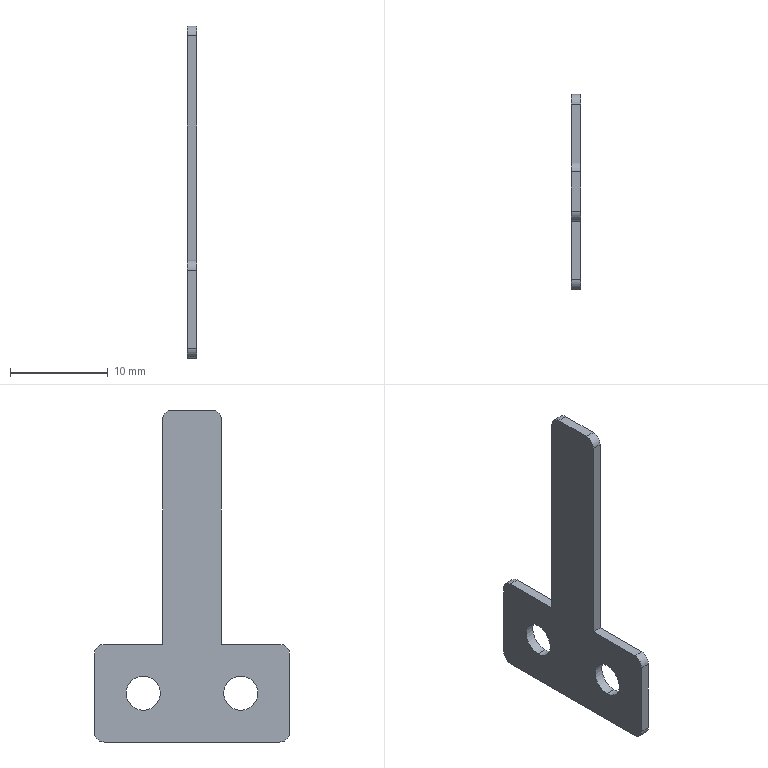Part | SolidWorks | features BaseBody 1 | 1 solid | 20 faces | box 1 x 20 x 34 mm | volume 323.47 mm3 | cylinder 10 | plane 10 | commonest cylinder face diameters 2 x6 3.5 x4
STEP:
#1=CARTESIAN_POINT('',(-1.,10.,-16.));
#2=VERTEX_POINT('',#1);
#3=CARTESIAN_POINT('',(-1.,9.,-17.));
#4=VERTEX_POINT('',#3);
#5=CARTESIAN_POINT('',(-1.,9.,-16.));
#6=DIRECTION('',(-1.,0.,0.));
#7=DIRECTION('',(0.,0.,-1.));
#8=AXIS2_PLACEMENT_3D('',#5,#6,#7);
#9=CIRCLE('',#8,1.);
#10=EDGE_CURVE('',#2,#4,#9,.T.);
#11=ORIENTED_EDGE('',*,*,#10,.F.);
#12=CARTESIAN_POINT('',(0.,10.,-16.));
#13=VERTEX_POINT('',#12);
#14=CARTESIAN_POINT('',(0.,10.,-16.));
#15=DIRECTION('',(-1.,0.,0.));
#16=VECTOR('',#15,1000.);
#17=LINE('',#14,#16);
#18=EDGE_CURVE('',#13,#2,#17,.T.);
#19=ORIENTED_EDGE('',*,*,#18,.F.);
#20=CARTESIAN_POINT('',(0.,9.,-17.));
#21=VERTEX_POINT('',#20);
#22=CARTESIAN_POINT('',(0.,9.,-16.));
#23=DIRECTION('',(1.,0.,0.));
#24=DIRECTION('',(0.,0.,-1.));
#25=AXIS2_PLACEMENT_3D('',#22,#23,#24);
#26=CIRCLE('',#25,1.);
#27=EDGE_CURVE('',#21,#13,#26,.T.);
#28=ORIENTED_EDGE('',*,*,#27,.F.);
#29=CARTESIAN_POINT('',(-1.,9.,-17.));
#30=DIRECTION('',(1.,0.,0.));
#31=VECTOR('',#30,1000.);
#32=LINE('',#29,#31);
#33=EDGE_CURVE('',#4,#21,#32,.T.);
#34=ORIENTED_EDGE('',*,*,#33,.F.);
#35=EDGE_LOOP('',(#11,#19,#28,#34));
#36=FACE_OUTER_BOUND('',#35,.T.);
#37=CARTESIAN_POINT('',(-1.,9.,-16.));
#38=DIRECTION('',(1.,0.,0.));
#39=DIRECTION('',(0.,0.,-1.));
#40=AXIS2_PLACEMENT_3D('',#37,#38,#39);
#41=CYLINDRICAL_SURFACE('',#40,1.);
#42=ADVANCED_FACE('',(#36),#41,.T.);
#43=CARTESIAN_POINT('',(-1.,9.,-7.));
#44=VERTEX_POINT('',#43);
#45=CARTESIAN_POINT('',(-1.,10.,-8.));
#46=VERTEX_POINT('',#45);
#47=CARTESIAN_POINT('',(-1.,9.,-8.));
#48=DIRECTION('',(-1.,0.,0.));
#49=DIRECTION('',(0.,0.,-1.));
#50=AXIS2_PLACEMENT_3D('',#47,#48,#49);
#51=CIRCLE('',#50,1.);
#52=EDGE_CURVE('',#44,#46,#51,.T.);
#53=ORIENTED_EDGE('',*,*,#52,.F.);
#54=CARTESIAN_POINT('',(0.,9.,-7.));
#55=VERTEX_POINT('',#54);
#56=CARTESIAN_POINT('',(-1.,9.,-7.));
#57=DIRECTION('',(-1.,0.,0.));
#58=VECTOR('',#57,1000.);
#59=LINE('',#56,#58);
#60=EDGE_CURVE('',#55,#44,#59,.T.);
#61=ORIENTED_EDGE('',*,*,#60,.F.);
#62=CARTESIAN_POINT('',(0.,10.,-8.));
#63=VERTEX_POINT('',#62);
#64=CARTESIAN_POINT('',(0.,9.,-8.));
#65=DIRECTION('',(1.,0.,0.));
#66=DIRECTION('',(0.,0.,-1.));
#67=AXIS2_PLACEMENT_3D('',#64,#65,#66);
#68=CIRCLE('',#67,1.);
#69=EDGE_CURVE('',#63,#55,#68,.T.);
#70=ORIENTED_EDGE('',*,*,#69,.F.);
#71=CARTESIAN_POINT('',(0.,10.,-8.));
#72=DIRECTION('',(1.,0.,0.));
#73=VECTOR('',#72,1000.);
#74=LINE('',#71,#73);
#75=EDGE_CURVE('',#46,#63,#74,.T.);
#76=ORIENTED_EDGE('',*,*,#75,.F.);
#77=EDGE_LOOP('',(#53,#61,#70,#76));
#78=FACE_OUTER_BOUND('',#77,.T.);
#79=CARTESIAN_POINT('',(0.,9.,-8.));
#80=DIRECTION('',(-1.,0.,0.));
#81=DIRECTION('',(0.,0.,1.));
#82=AXIS2_PLACEMENT_3D('',#79,#80,#81);
#83=CYLINDRICAL_SURFACE('',#82,1.);
#84=ADVANCED_FACE('',(#78),#83,.T.);
#85=CARTESIAN_POINT('',(-1.,2.,17.));
#86=VERTEX_POINT('',#85);
#87=CARTESIAN_POINT('',(-1.,3.,16.));
#88=VERTEX_POINT('',#87);
#89=CARTESIAN_POINT('',(-1.,2.,16.));
#90=DIRECTION('',(-1.,0.,0.));
#91=DIRECTION('',(0.,0.,-1.));
#92=AXIS2_PLACEMENT_3D('',#89,#90,#91);
#93=CIRCLE('',#92,1.);
#94=EDGE_CURVE('',#86,#88,#93,.T.);
#95=ORIENTED_EDGE('',*,*,#94,.F.);
#96=CARTESIAN_POINT('',(0.,2.,17.));
#97=VERTEX_POINT('',#96);
#98=CARTESIAN_POINT('',(-1.,2.,17.));
#99=DIRECTION('',(-1.,0.,0.));
#100=VECTOR('',#99,1000.);
#101=LINE('',#98,#100);
#102=EDGE_CURVE('',#97,#86,#101,.T.);
#103=ORIENTED_EDGE('',*,*,#102,.F.);
#104=CARTESIAN_POINT('',(0.,3.,16.));
#105=VERTEX_POINT('',#104);
#106=CARTESIAN_POINT('',(0.,2.,16.));
#107=DIRECTION('',(1.,0.,0.));
#108=DIRECTION('',(0.,0.,-1.));
#109=AXIS2_PLACEMENT_3D('',#106,#107,#108);
#110=CIRCLE('',#109,1.);
#111=EDGE_CURVE('',#105,#97,#110,.T.);
#112=ORIENTED_EDGE('',*,*,#111,.F.);
#113=CARTESIAN_POINT('',(0.,3.,16.));
#114=DIRECTION('',(1.,0.,0.));
#115=VECTOR('',#114,1000.);
#116=LINE('',#113,#115);
#117=EDGE_CURVE('',#88,#105,#116,.T.);
#118=ORIENTED_EDGE('',*,*,#117,.F.);
#119=EDGE_LOOP('',(#95,#103,#112,#118));
#120=FACE_OUTER_BOUND('',#119,.T.);
#121=CARTESIAN_POINT('',(-26.,2.,16.));
#122=DIRECTION('',(-1.,0.,0.));
#123=DIRECTION('',(0.,0.,1.));
#124=AXIS2_PLACEMENT_3D('',#121,#122,#123);
#125=CYLINDRICAL_SURFACE('',#124,1.);
#126=ADVANCED_FACE('',(#120),#125,.T.);
#127=CARTESIAN_POINT('',(-1.,-3.,16.));
#128=VERTEX_POINT('',#127);
#129=CARTESIAN_POINT('',(-1.,-2.,17.));
#130=VERTEX_POINT('',#129);
#131=CARTESIAN_POINT('',(-1.,-2.,16.));
#132=DIRECTION('',(-1.,0.,0.));
#133=DIRECTION('',(0.,0.,-1.));
#134=AXIS2_PLACEMENT_3D('',#131,#132,#133);
#135=CIRCLE('',#134,1.);
#136=EDGE_CURVE('',#128,#130,#135,.T.);
#137=ORIENTED_EDGE('',*,*,#136,.F.);
#138=CARTESIAN_POINT('',(0.,-3.,16.));
#139=VERTEX_POINT('',#138);
#140=CARTESIAN_POINT('',(-1.,-3.,16.));
#141=DIRECTION('',(-1.,0.,0.));
#142=VECTOR('',#141,1000.);
#143=LINE('',#140,#142);
#144=EDGE_CURVE('',#139,#128,#143,.T.);
#145=ORIENTED_EDGE('',*,*,#144,.F.);
#146=CARTESIAN_POINT('',(0.,-2.,17.));
#147=VERTEX_POINT('',#146);
#148=CARTESIAN_POINT('',(0.,-2.,16.));
#149=DIRECTION('',(1.,0.,0.));
#150=DIRECTION('',(0.,0.,-1.));
#151=AXIS2_PLACEMENT_3D('',#148,#149,#150);
#152=CIRCLE('',#151,1.);
#153=EDGE_CURVE('',#147,#139,#152,.T.);
#154=ORIENTED_EDGE('',*,*,#153,.F.);
#155=CARTESIAN_POINT('',(0.,-2.,17.));
#156=DIRECTION('',(1.,0.,0.));
#157=VECTOR('',#156,1000.);
#158=LINE('',#155,#157);
#159=EDGE_CURVE('',#130,#147,#158,.T.);
#160=ORIENTED_EDGE('',*,*,#159,.F.);
#161=EDGE_LOOP('',(#137,#145,#154,#160));
#162=FACE_OUTER_BOUND('',#161,.T.);
#163=CARTESIAN_POINT('',(0.,-2.,16.));
#164=DIRECTION('',(-1.,0.,0.));
#165=DIRECTION('',(0.,0.,1.));
#166=AXIS2_PLACEMENT_3D('',#163,#164,#165);
#167=CYLINDRICAL_SURFACE('',#166,1.);
#168=ADVANCED_FACE('',(#162),#167,.T.);
#169=CARTESIAN_POINT('',(-1.,-10.,-8.));
#170=VERTEX_POINT('',#169);
#171=CARTESIAN_POINT('',(-1.,-9.,-7.));
#172=VERTEX_POINT('',#171);
#173=CARTESIAN_POINT('',(-1.,-9.,-8.));
#174=DIRECTION('',(-1.,0.,0.));
#175=DIRECTION('',(0.,0.,-1.));
#176=AXIS2_PLACEMENT_3D('',#173,#174,#175);
#177=CIRCLE('',#176,1.);
#178=EDGE_CURVE('',#170,#172,#177,.T.);
#179=ORIENTED_EDGE('',*,*,#178,.F.);
#180=CARTESIAN_POINT('',(0.,-10.,-8.));
#181=VERTEX_POINT('',#180);
#182=CARTESIAN_POINT('',(0.,-10.,-8.));
#183=DIRECTION('',(-1.,0.,0.));
#184=VECTOR('',#183,1000.);
#185=LINE('',#182,#184);
#186=EDGE_CURVE('',#181,#170,#185,.T.);
#187=ORIENTED_EDGE('',*,*,#186,.F.);
#188=CARTESIAN_POINT('',(0.,-9.,-7.));
#189=VERTEX_POINT('',#188);
#190=CARTESIAN_POINT('',(0.,-9.,-8.));
#191=DIRECTION('',(1.,0.,0.));
#192=DIRECTION('',(0.,0.,-1.));
#193=AXIS2_PLACEMENT_3D('',#190,#191,#192);
#194=CIRCLE('',#193,1.);
#195=EDGE_CURVE('',#189,#181,#194,.T.);
#196=ORIENTED_EDGE('',*,*,#195,.F.);
#197=CARTESIAN_POINT('',(-26.,-9.,-7.));
#198=DIRECTION('',(1.,0.,0.));
#199=VECTOR('',#198,1000.);
#200=LINE('',#197,#199);
#201=EDGE_CURVE('',#172,#189,#200,.T.);
#202=ORIENTED_EDGE('',*,*,#201,.F.);
#203=EDGE_LOOP('',(#179,#187,#196,#202));
#204=FACE_OUTER_BOUND('',#203,.T.);
#205=CARTESIAN_POINT('',(-26.,-9.,-8.));
#206=DIRECTION('',(1.,0.,0.));
#207=DIRECTION('',(0.,0.,-1.));
#208=AXIS2_PLACEMENT_3D('',#205,#206,#207);
#209=CYLINDRICAL_SURFACE('',#208,1.);
#210=ADVANCED_FACE('',(#204),#209,.T.);
#211=CARTESIAN_POINT('',(-1.,-9.,-17.));
#212=VERTEX_POINT('',#211);
#213=CARTESIAN_POINT('',(-1.,-10.,-16.));
#214=VERTEX_POINT('',#213);
#215=CARTESIAN_POINT('',(-1.,-9.,-16.));
#216=DIRECTION('',(-1.,0.,0.));
#217=DIRECTION('',(0.,0.,-1.));
#218=AXIS2_PLACEMENT_3D('',#215,#216,#217);
#219=CIRCLE('',#218,1.);
#220=EDGE_CURVE('',#212,#214,#219,.T.);
#221=ORIENTED_EDGE('',*,*,#220,.F.);
#222=CARTESIAN_POINT('',(0.,-9.,-17.));
#223=VERTEX_POINT('',#222);
#224=CARTESIAN_POINT('',(-1.,-9.,-17.));
#225=DIRECTION('',(-1.,0.,0.));
#226=VECTOR('',#225,1000.);
#227=LINE('',#224,#226);
#228=EDGE_CURVE('',#223,#212,#227,.T.);
#229=ORIENTED_EDGE('',*,*,#228,.F.);
#230=CARTESIAN_POINT('',(0.,-10.,-16.));
#231=VERTEX_POINT('',#230);
#232=CARTESIAN_POINT('',(0.,-9.,-16.));
#233=DIRECTION('',(1.,0.,0.));
#234=DIRECTION('',(0.,0.,-1.));
#235=AXIS2_PLACEMENT_3D('',#232,#233,#234);
#236=CIRCLE('',#235,1.);
#237=EDGE_CURVE('',#231,#223,#236,.T.);
#238=ORIENTED_EDGE('',*,*,#237,.F.);
#239=CARTESIAN_POINT('',(0.,-10.,-16.));
#240=DIRECTION('',(1.,0.,0.));
#241=VECTOR('',#240,1000.);
#242=LINE('',#239,#241);
#243=EDGE_CURVE('',#214,#231,#242,.T.);
#244=ORIENTED_EDGE('',*,*,#243,.F.);
#245=EDGE_LOOP('',(#221,#229,#238,#244));
#246=FACE_OUTER_BOUND('',#245,.T.);
#247=CARTESIAN_POINT('',(0.,-9.,-16.));
#248=DIRECTION('',(-1.,0.,0.));
#249=DIRECTION('',(0.,0.,1.));
#250=AXIS2_PLACEMENT_3D('',#247,#248,#249);
#251=CYLINDRICAL_SURFACE('',#250,1.);
#252=ADVANCED_FACE('',(#246),#251,.T.);
#253=CARTESIAN_POINT('',(-1.,3.,-7.));
#254=VERTEX_POINT('',#253);
#255=CARTESIAN_POINT('',(-1.,3.,17.));
#256=DIRECTION('',(0.,0.,1.));
#257=VECTOR('',#256,1000.);
#258=LINE('',#255,#257);
#259=EDGE_CURVE('',#254,#88,#258,.T.);
#260=ORIENTED_EDGE('',*,*,#259,.T.);
#261=ORIENTED_EDGE('',*,*,#117,.T.);
#262=CARTESIAN_POINT('',(0.,3.,-7.));
#263=VERTEX_POINT('',#262);
#264=CARTESIAN_POINT('',(0.,3.,17.));
#265=DIRECTION('',(0.,0.,-1.));
#266=VECTOR('',#265,1000.);
#267=LINE('',#264,#266);
#268=EDGE_CURVE('',#105,#263,#267,.T.);
#269=ORIENTED_EDGE('',*,*,#268,.T.);
#270=CARTESIAN_POINT('',(-26.,3.,-7.));
#271=DIRECTION('',(1.,0.,0.));
#272=VECTOR('',#271,1000.);
#273=LINE('',#270,#272);
#274=EDGE_CURVE('',#254,#263,#273,.T.);
#275=ORIENTED_EDGE('',*,*,#274,.F.);
#276=EDGE_LOOP('',(#260,#261,#269,#275));
#277=FACE_OUTER_BOUND('',#276,.T.);
#278=CARTESIAN_POINT('',(-26.,3.,17.));
#279=DIRECTION('',(0.,-1.,0.));
#280=DIRECTION('',(0.,0.,-1.));
#281=AXIS2_PLACEMENT_3D('',#278,#279,#280);
#282=PLANE('',#281);
#283=ADVANCED_FACE('',(#277),#282,.F.);
#284=CARTESIAN_POINT('',(0.,10.,-7.));
#285=DIRECTION('',(0.,1.,0.));
#286=VECTOR('',#285,1000.);
#287=LINE('',#284,#286);
#288=EDGE_CURVE('',#263,#55,#287,.T.);
#289=ORIENTED_EDGE('',*,*,#288,.T.);
#290=ORIENTED_EDGE('',*,*,#60,.T.);
#291=CARTESIAN_POINT('',(-1.,10.,-7.));
#292=DIRECTION('',(0.,-1.,0.));
#293=VECTOR('',#292,1000.);
#294=LINE('',#291,#293);
#295=EDGE_CURVE('',#44,#254,#294,.T.);
#296=ORIENTED_EDGE('',*,*,#295,.T.);
#297=ORIENTED_EDGE('',*,*,#274,.T.);
#298=EDGE_LOOP('',(#289,#290,#296,#297));
#299=FACE_OUTER_BOUND('',#298,.T.);
#300=CARTESIAN_POINT('',(-26.,10.,-7.));
#301=DIRECTION('',(0.,0.,-1.));
#302=DIRECTION('',(-1.,0.,0.));
#303=AXIS2_PLACEMENT_3D('',#300,#301,#302);
#304=PLANE('',#303);
#305=ADVANCED_FACE('',(#299),#304,.F.);
#306=CARTESIAN_POINT('',(-1.,-3.,-7.));
#307=VERTEX_POINT('',#306);
#308=CARTESIAN_POINT('',(-1.,-10.,-7.));
#309=DIRECTION('',(0.,-1.,0.));
#310=VECTOR('',#309,1000.);
#311=LINE('',#308,#310);
#312=EDGE_CURVE('',#307,#172,#311,.T.);
#313=ORIENTED_EDGE('',*,*,#312,.T.);
#314=ORIENTED_EDGE('',*,*,#201,.T.);
#315=CARTESIAN_POINT('',(0.,-3.,-7.));
#316=VERTEX_POINT('',#315);
#317=CARTESIAN_POINT('',(0.,-10.,-7.));
#318=DIRECTION('',(0.,1.,0.));
#319=VECTOR('',#318,1000.);
#320=LINE('',#317,#319);
#321=EDGE_CURVE('',#189,#316,#320,.T.);
#322=ORIENTED_EDGE('',*,*,#321,.T.);
#323=CARTESIAN_POINT('',(-26.,-3.,-7.));
#324=DIRECTION('',(1.,0.,0.));
#325=VECTOR('',#324,1000.);
#326=LINE('',#323,#325);
#327=EDGE_CURVE('',#307,#316,#326,.T.);
#328=ORIENTED_EDGE('',*,*,#327,.F.);
#329=EDGE_LOOP('',(#313,#314,#322,#328));
#330=FACE_OUTER_BOUND('',#329,.T.);
#331=CARTESIAN_POINT('',(-26.,-10.,-7.));
#332=DIRECTION('',(0.,0.,-1.));
#333=DIRECTION('',(-1.,0.,0.));
#334=AXIS2_PLACEMENT_3D('',#331,#332,#333);
#335=PLANE('',#334);
#336=ADVANCED_FACE('',(#330),#335,.F.);
#337=CARTESIAN_POINT('',(0.,-3.,17.));
#338=DIRECTION('',(0.,0.,1.));
#339=VECTOR('',#338,1000.);
#340=LINE('',#337,#339);
#341=EDGE_CURVE('',#316,#139,#340,.T.);
#342=ORIENTED_EDGE('',*,*,#341,.T.);
#343=ORIENTED_EDGE('',*,*,#144,.T.);
#344=CARTESIAN_POINT('',(-1.,-3.,17.));
#345=DIRECTION('',(0.,0.,-1.));
#346=VECTOR('',#345,1000.);
#347=LINE('',#344,#346);
#348=EDGE_CURVE('',#128,#307,#347,.T.);
#349=ORIENTED_EDGE('',*,*,#348,.T.);
#350=ORIENTED_EDGE('',*,*,#327,.T.);
#351=EDGE_LOOP('',(#342,#343,#349,#350));
#352=FACE_OUTER_BOUND('',#351,.T.);
#353=CARTESIAN_POINT('',(-26.,-3.,17.));
#354=DIRECTION('',(0.,1.,0.));
#355=DIRECTION('',(0.,0.,-1.));
#356=AXIS2_PLACEMENT_3D('',#353,#354,#355);
#357=PLANE('',#356);
#358=ADVANCED_FACE('',(#352),#357,.F.);
#359=CARTESIAN_POINT('',(-1.,5.,-10.25));
#360=VERTEX_POINT('',#359);
#361=CARTESIAN_POINT('',(0.,5.,-10.25));
#362=VERTEX_POINT('',#361);
#363=CARTESIAN_POINT('',(0.,5.,-10.25));
#364=DIRECTION('',(1.,0.,0.));
#365=VECTOR('',#364,1000.);
#366=LINE('',#363,#365);
#367=EDGE_CURVE('',#360,#362,#366,.T.);
#368=ORIENTED_EDGE('',*,*,#367,.F.);
#369=CARTESIAN_POINT('',(-1.,5.,-13.75));
#370=VERTEX_POINT('',#369);
#371=CARTESIAN_POINT('',(-1.,5.,-12.));
#372=DIRECTION('',(1.,0.,0.));
#373=DIRECTION('',(0.,0.,-1.));
#374=AXIS2_PLACEMENT_3D('',#371,#372,#373);
#375=CIRCLE('',#374,1.75);
#376=EDGE_CURVE('',#370,#360,#375,.T.);
#377=ORIENTED_EDGE('',*,*,#376,.F.);
#378=CARTESIAN_POINT('',(0.,5.,-13.75));
#379=VERTEX_POINT('',#378);
#380=CARTESIAN_POINT('',(0.,5.,-13.75));
#381=DIRECTION('',(1.,0.,0.));
#382=VECTOR('',#381,1000.);
#383=LINE('',#380,#382);
#384=EDGE_CURVE('',#370,#379,#383,.T.);
#385=ORIENTED_EDGE('',*,*,#384,.T.);
#386=CARTESIAN_POINT('',(0.,5.,-12.));
#387=DIRECTION('',(1.,0.,0.));
#388=DIRECTION('',(0.,0.,-1.));
#389=AXIS2_PLACEMENT_3D('',#386,#387,#388);
#390=CIRCLE('',#389,1.75);
#391=EDGE_CURVE('',#379,#362,#390,.T.);
#392=ORIENTED_EDGE('',*,*,#391,.T.);
#393=EDGE_LOOP('',(#368,#377,#385,#392));
#394=FACE_OUTER_BOUND('',#393,.T.);
#395=CARTESIAN_POINT('',(0.,5.,-12.));
#396=DIRECTION('',(1.,0.,0.));
#397=DIRECTION('',(0.,0.,-1.));
#398=AXIS2_PLACEMENT_3D('',#395,#396,#397);
#399=CYLINDRICAL_SURFACE('',#398,1.75);
#400=ADVANCED_FACE('',(#394),#399,.F.);
#401=CARTESIAN_POINT('',(-1.,-5.,-10.25));
#402=VERTEX_POINT('',#401);
#403=CARTESIAN_POINT('',(0.,-5.,-10.25));
#404=VERTEX_POINT('',#403);
#405=CARTESIAN_POINT('',(0.,-5.,-10.25));
#406=DIRECTION('',(1.,0.,0.));
#407=VECTOR('',#406,1000.);
#408=LINE('',#405,#407);
#409=EDGE_CURVE('',#402,#404,#408,.T.);
#410=ORIENTED_EDGE('',*,*,#409,.F.);
#411=CARTESIAN_POINT('',(-1.,-5.,-13.75));
#412=VERTEX_POINT('',#411);
#413=CARTESIAN_POINT('',(-1.,-5.,-12.));
#414=DIRECTION('',(1.,0.,0.));
#415=DIRECTION('',(0.,0.,-1.));
#416=AXIS2_PLACEMENT_3D('',#413,#414,#415);
#417=CIRCLE('',#416,1.75);
#418=EDGE_CURVE('',#412,#402,#417,.T.);
#419=ORIENTED_EDGE('',*,*,#418,.F.);
#420=CARTESIAN_POINT('',(0.,-5.,-13.75));
#421=VERTEX_POINT('',#420);
#422=CARTESIAN_POINT('',(0.,-5.,-13.75));
#423=DIRECTION('',(1.,0.,0.));
#424=VECTOR('',#423,1000.);
#425=LINE('',#422,#424);
#426=EDGE_CURVE('',#412,#421,#425,.T.);
#427=ORIENTED_EDGE('',*,*,#426,.T.);
#428=CARTESIAN_POINT('',(0.,-5.,-12.));
#429=DIRECTION('',(1.,0.,0.));
#430=DIRECTION('',(0.,0.,-1.));
#431=AXIS2_PLACEMENT_3D('',#428,#429,#430);
#432=CIRCLE('',#431,1.75);
#433=EDGE_CURVE('',#421,#404,#432,.T.);
#434=ORIENTED_EDGE('',*,*,#433,.T.);
#435=EDGE_LOOP('',(#410,#419,#427,#434));
#436=FACE_OUTER_BOUND('',#435,.T.);
#437=CARTESIAN_POINT('',(0.,-5.,-12.));
#438=DIRECTION('',(1.,0.,0.));
#439=DIRECTION('',(0.,0.,-1.));
#440=AXIS2_PLACEMENT_3D('',#437,#438,#439);
#441=CYLINDRICAL_SURFACE('',#440,1.75);
#442=ADVANCED_FACE('',(#436),#441,.F.);
#443=CARTESIAN_POINT('',(-1.,-10.,-17.));
#444=DIRECTION('',(0.,0.,1.));
#445=VECTOR('',#444,1000.);
#446=LINE('',#443,#445);
#447=EDGE_CURVE('',#214,#170,#446,.T.);
#448=ORIENTED_EDGE('',*,*,#447,.F.);
#449=ORIENTED_EDGE('',*,*,#243,.T.);
#450=CARTESIAN_POINT('',(0.,-10.,-17.));
#451=DIRECTION('',(0.,0.,1.));
#452=VECTOR('',#451,1000.);
#453=LINE('',#450,#452);
#454=EDGE_CURVE('',#231,#181,#453,.T.);
#455=ORIENTED_EDGE('',*,*,#454,.T.);
#456=ORIENTED_EDGE('',*,*,#186,.T.);
#457=EDGE_LOOP('',(#448,#449,#455,#456));
#458=FACE_OUTER_BOUND('',#457,.T.);
#459=CARTESIAN_POINT('',(0.,-10.,0.));
#460=DIRECTION('',(0.,1.,0.));
#461=DIRECTION('',(1.,0.,0.));
#462=AXIS2_PLACEMENT_3D('',#459,#460,#461);
#463=PLANE('',#462);
#464=ADVANCED_FACE('',(#458),#463,.F.);
#465=CARTESIAN_POINT('',(-1.,10.,-17.));
#466=DIRECTION('',(0.,0.,1.));
#467=VECTOR('',#466,1000.);
#468=LINE('',#465,#467);
#469=EDGE_CURVE('',#2,#46,#468,.T.);
#470=ORIENTED_EDGE('',*,*,#469,.T.);
#471=ORIENTED_EDGE('',*,*,#75,.T.);
#472=CARTESIAN_POINT('',(0.,10.,-17.));
#473=DIRECTION('',(0.,0.,1.));
#474=VECTOR('',#473,1000.);
#475=LINE('',#472,#474);
#476=EDGE_CURVE('',#13,#63,#475,.T.);
#477=ORIENTED_EDGE('',*,*,#476,.F.);
#478=ORIENTED_EDGE('',*,*,#18,.T.);
#479=EDGE_LOOP('',(#470,#471,#477,#478));
#480=FACE_OUTER_BOUND('',#479,.T.);
#481=CARTESIAN_POINT('',(0.,10.,0.));
#482=DIRECTION('',(0.,1.,0.));
#483=DIRECTION('',(1.,0.,0.));
#484=AXIS2_PLACEMENT_3D('',#481,#482,#483);
#485=PLANE('',#484);
#486=ADVANCED_FACE('',(#480),#485,.T.);
#487=CARTESIAN_POINT('',(0.,10.,-17.));
#488=DIRECTION('',(0.,-1.,0.));
#489=VECTOR('',#488,1000.);
#490=LINE('',#487,#489);
#491=EDGE_CURVE('',#21,#223,#490,.T.);
#492=ORIENTED_EDGE('',*,*,#491,.T.);
#493=ORIENTED_EDGE('',*,*,#228,.T.);
#494=CARTESIAN_POINT('',(-1.,10.,-17.));
#495=DIRECTION('',(0.,-1.,0.));
#496=VECTOR('',#495,1000.);
#497=LINE('',#494,#496);
#498=EDGE_CURVE('',#4,#212,#497,.T.);
#499=ORIENTED_EDGE('',*,*,#498,.F.);
#500=ORIENTED_EDGE('',*,*,#33,.T.);
#501=EDGE_LOOP('',(#492,#493,#499,#500));
#502=FACE_OUTER_BOUND('',#501,.T.);
#503=CARTESIAN_POINT('',(-1.,10.,-17.));
#504=DIRECTION('',(0.,0.,-1.));
#505=DIRECTION('',(0.,-1.,0.));
#506=AXIS2_PLACEMENT_3D('',#503,#504,#505);
#507=PLANE('',#506);
#508=ADVANCED_FACE('',(#502),#507,.T.);
#509=ORIENTED_EDGE('',*,*,#433,.F.);
#510=CARTESIAN_POINT('',(0.,-5.,-12.));
#511=DIRECTION('',(1.,0.,0.));
#512=DIRECTION('',(0.,0.,-1.));
#513=AXIS2_PLACEMENT_3D('',#510,#511,#512);
#514=CIRCLE('',#513,1.75);
#515=EDGE_CURVE('',#404,#421,#514,.T.);
#516=ORIENTED_EDGE('',*,*,#515,.F.);
#517=EDGE_LOOP('',(#509,#516));
#518=FACE_BOUND('',#517,.T.);
#519=ORIENTED_EDGE('',*,*,#391,.F.);
#520=CARTESIAN_POINT('',(0.,5.,-12.));
#521=DIRECTION('',(1.,0.,0.));
#522=DIRECTION('',(0.,0.,-1.));
#523=AXIS2_PLACEMENT_3D('',#520,#521,#522);
#524=CIRCLE('',#523,1.75);
#525=EDGE_CURVE('',#362,#379,#524,.T.);
#526=ORIENTED_EDGE('',*,*,#525,.F.);
#527=EDGE_LOOP('',(#519,#526));
#528=FACE_BOUND('',#527,.T.);
#529=ORIENTED_EDGE('',*,*,#454,.F.);
#530=ORIENTED_EDGE('',*,*,#237,.T.);
#531=ORIENTED_EDGE('',*,*,#491,.F.);
#532=ORIENTED_EDGE('',*,*,#27,.T.);
#533=ORIENTED_EDGE('',*,*,#476,.T.);
#534=ORIENTED_EDGE('',*,*,#69,.T.);
#535=ORIENTED_EDGE('',*,*,#288,.F.);
#536=ORIENTED_EDGE('',*,*,#268,.F.);
#537=ORIENTED_EDGE('',*,*,#111,.T.);
#538=CARTESIAN_POINT('',(0.,10.,17.));
#539=DIRECTION('',(0.,-1.,0.));
#540=VECTOR('',#539,1000.);
#541=LINE('',#538,#540);
#542=EDGE_CURVE('',#97,#147,#541,.T.);
#543=ORIENTED_EDGE('',*,*,#542,.T.);
#544=ORIENTED_EDGE('',*,*,#153,.T.);
#545=ORIENTED_EDGE('',*,*,#341,.F.);
#546=ORIENTED_EDGE('',*,*,#321,.F.);
#547=ORIENTED_EDGE('',*,*,#195,.T.);
#548=EDGE_LOOP('',(#529,#530,#531,#532,#533,#534,#535,#536,#537,#543,#544,#545,#546,#547));
#549=FACE_OUTER_BOUND('',#548,.T.);
#550=CARTESIAN_POINT('',(0.,10.,-17.));
#551=DIRECTION('',(1.,0.,0.));
#552=DIRECTION('',(0.,1.,0.));
#553=AXIS2_PLACEMENT_3D('',#550,#551,#552);
#554=PLANE('',#553);
#555=ADVANCED_FACE('',(#518,#528,#549),#554,.T.);
#556=CARTESIAN_POINT('',(-1.,10.,17.));
#557=DIRECTION('',(0.,-1.,0.));
#558=VECTOR('',#557,1000.);
#559=LINE('',#556,#558);
#560=EDGE_CURVE('',#86,#130,#559,.T.);
#561=ORIENTED_EDGE('',*,*,#560,.T.);
#562=ORIENTED_EDGE('',*,*,#159,.T.);
#563=ORIENTED_EDGE('',*,*,#542,.F.);
#564=ORIENTED_EDGE('',*,*,#102,.T.);
#565=EDGE_LOOP('',(#561,#562,#563,#564));
#566=FACE_OUTER_BOUND('',#565,.T.);
#567=CARTESIAN_POINT('',(0.,10.,17.));
#568=DIRECTION('',(0.,0.,1.));
#569=DIRECTION('',(1.,0.,0.));
#570=AXIS2_PLACEMENT_3D('',#567,#568,#569);
#571=PLANE('',#570);
#572=ADVANCED_FACE('',(#566),#571,.T.);
#573=ORIENTED_EDGE('',*,*,#418,.T.);
#574=CARTESIAN_POINT('',(-1.,-5.,-12.));
#575=DIRECTION('',(1.,0.,0.));
#576=DIRECTION('',(0.,0.,-1.));
#577=AXIS2_PLACEMENT_3D('',#574,#575,#576);
#578=CIRCLE('',#577,1.75);
#579=EDGE_CURVE('',#402,#412,#578,.T.);
#580=ORIENTED_EDGE('',*,*,#579,.T.);
#581=EDGE_LOOP('',(#573,#580));
#582=FACE_BOUND('',#581,.T.);
#583=ORIENTED_EDGE('',*,*,#376,.T.);
#584=CARTESIAN_POINT('',(-1.,5.,-12.));
#585=DIRECTION('',(1.,0.,0.));
#586=DIRECTION('',(0.,0.,-1.));
#587=AXIS2_PLACEMENT_3D('',#584,#585,#586);
#588=CIRCLE('',#587,1.75);
#589=EDGE_CURVE('',#360,#370,#588,.T.);
#590=ORIENTED_EDGE('',*,*,#589,.T.);
#591=EDGE_LOOP('',(#583,#590));
#592=FACE_BOUND('',#591,.T.);
#593=ORIENTED_EDGE('',*,*,#498,.T.);
#594=ORIENTED_EDGE('',*,*,#220,.T.);
#595=ORIENTED_EDGE('',*,*,#447,.T.);
#596=ORIENTED_EDGE('',*,*,#178,.T.);
#597=ORIENTED_EDGE('',*,*,#312,.F.);
#598=ORIENTED_EDGE('',*,*,#348,.F.);
#599=ORIENTED_EDGE('',*,*,#136,.T.);
#600=ORIENTED_EDGE('',*,*,#560,.F.);
#601=ORIENTED_EDGE('',*,*,#94,.T.);
#602=ORIENTED_EDGE('',*,*,#259,.F.);
#603=ORIENTED_EDGE('',*,*,#295,.F.);
#604=ORIENTED_EDGE('',*,*,#52,.T.);
#605=ORIENTED_EDGE('',*,*,#469,.F.);
#606=ORIENTED_EDGE('',*,*,#10,.T.);
#607=EDGE_LOOP('',(#593,#594,#595,#596,#597,#598,#599,#600,#601,#602,#603,#604,#605,#606));
#608=FACE_OUTER_BOUND('',#607,.T.);
#609=CARTESIAN_POINT('',(-1.,10.,-17.));
#610=DIRECTION('',(1.,0.,0.));
#611=DIRECTION('',(0.,1.,0.));
#612=AXIS2_PLACEMENT_3D('',#609,#610,#611);
#613=PLANE('',#612);
#614=ADVANCED_FACE('',(#582,#592,#608),#613,.F.);
#615=ORIENTED_EDGE('',*,*,#579,.F.);
#616=ORIENTED_EDGE('',*,*,#409,.T.);
#617=ORIENTED_EDGE('',*,*,#515,.T.);
#618=ORIENTED_EDGE('',*,*,#426,.F.);
#619=EDGE_LOOP('',(#615,#616,#617,#618));
#620=FACE_OUTER_BOUND('',#619,.T.);
#621=CARTESIAN_POINT('',(0.,-5.,-12.));
#622=DIRECTION('',(1.,0.,0.));
#623=DIRECTION('',(0.,0.,-1.));
#624=AXIS2_PLACEMENT_3D('',#621,#622,#623);
#625=CYLINDRICAL_SURFACE('',#624,1.75);
#626=ADVANCED_FACE('',(#620),#625,.F.);
#627=ORIENTED_EDGE('',*,*,#589,.F.);
#628=ORIENTED_EDGE('',*,*,#367,.T.);
#629=ORIENTED_EDGE('',*,*,#525,.T.);
#630=ORIENTED_EDGE('',*,*,#384,.F.);
#631=EDGE_LOOP('',(#627,#628,#629,#630));
#632=FACE_OUTER_BOUND('',#631,.T.);
#633=CARTESIAN_POINT('',(0.,5.,-12.));
#634=DIRECTION('',(1.,0.,0.));
#635=DIRECTION('',(0.,0.,-1.));
#636=AXIS2_PLACEMENT_3D('',#633,#634,#635);
#637=CYLINDRICAL_SURFACE('',#636,1.75);
#638=ADVANCED_FACE('',(#632),#637,.F.);
#639=CLOSED_SHELL('',(#42,#84,#126,#168,#210,#252,#283,#305,#336,#358,#400,#442,#464,#486,#508,#555,#572,#614,#626,#638));
#640=MANIFOLD_SOLID_BREP('',#639);
#641=CARTESIAN_POINT('',(0.,0.,0.));
#642=DIRECTION('',(0.,0.,1.));
#643=DIRECTION('',(1.,0.,0.));
#644=AXIS2_PLACEMENT_3D('',#641,#642,#643);
#645=(LENGTH_UNIT()NAMED_UNIT(*)SI_UNIT(.MILLI.,.METRE.));
#646=UNCERTAINTY_MEASURE_WITH_UNIT(LENGTH_MEASURE(0.00001),#645,'','');
#647=(NAMED_UNIT(*)PLANE_ANGLE_UNIT()SI_UNIT($,.RADIAN.));
#648=(NAMED_UNIT(*)SI_UNIT($,.STERADIAN.)SOLID_ANGLE_UNIT());
#649=(GEOMETRIC_REPRESENTATION_CONTEXT(3)GLOBAL_UNCERTAINTY_ASSIGNED_CONTEXT((#646))GLOBAL_UNIT_ASSIGNED_CONTEXT((#645,#647,#648))REPRESENTATION_CONTEXT('',''));
#650=ADVANCED_BREP_SHAPE_REPRESENTATION('',(#640,#644),#649);